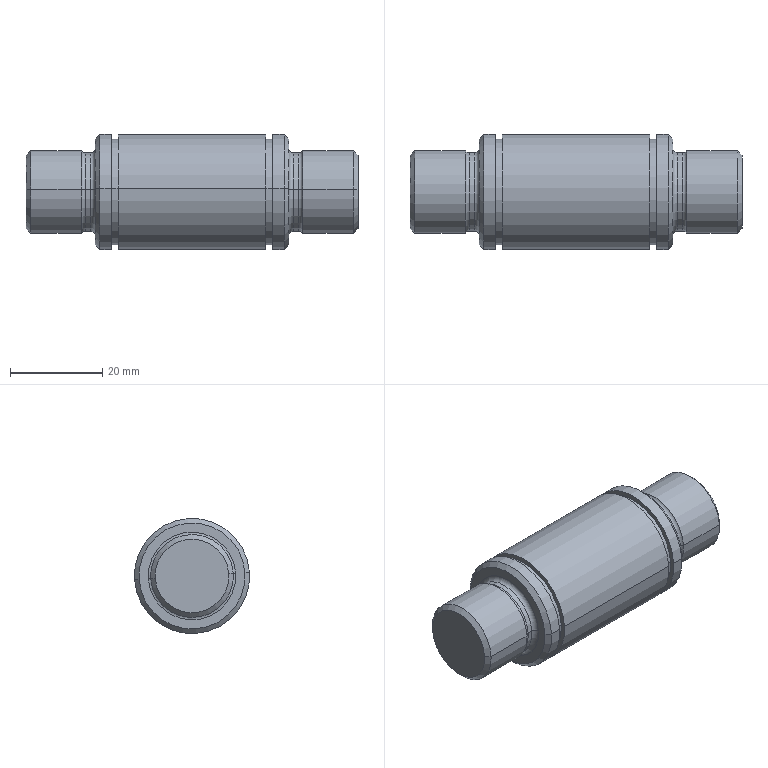Part | NX | features BREP 1 | 1 solid | 42 faces | box 72 x 25 x 25 mm | volume 27766 mm3 | cylinder 18 | cone 8 | torus 8 | plane 8 | commonest cylinder face diameters 25 x6 17 x4 18 x4 23 x4
STEP:
#1=CARTESIAN_POINT('',(-570.855,-69.053,-19.134));
#2=VERTEX_POINT('',#1);
#3=CARTESIAN_POINT('',(-570.855,-44.108,-20.797));
#4=VERTEX_POINT('',#3);
#5=CARTESIAN_POINT('',(-570.855,-56.581,-19.965));
#6=DIRECTION('',(1.,0.,0.));
#7=DIRECTION('',(0.,0.9978,-0.06652));
#8=AXIS2_PLACEMENT_3D('',#5,#6,#7);
#9=CIRCLE('',#8,12.5);
#10=EDGE_CURVE('',#2,#4,#9,.T.);
#11=ORIENTED_EDGE('',*,*,#10,.T.);
#12=CARTESIAN_POINT('',(-568.355,-44.108,-20.797));
#13=VERTEX_POINT('',#12);
#14=CARTESIAN_POINT('',(-609.355,-44.108,-20.797));
#15=DIRECTION('',(1.,0.,0.));
#16=VECTOR('',#15,1000.);
#17=LINE('',#14,#16);
#18=EDGE_CURVE('',#13,#4,#17,.F.);
#19=ORIENTED_EDGE('',*,*,#18,.F.);
#20=CARTESIAN_POINT('',(-568.355,-69.053,-19.134));
#21=VERTEX_POINT('',#20);
#22=CARTESIAN_POINT('',(-568.355,-56.581,-19.965));
#23=DIRECTION('',(-1.,0.,0.));
#24=DIRECTION('',(0.,-0.9978,0.06652));
#25=AXIS2_PLACEMENT_3D('',#22,#23,#24);
#26=CIRCLE('',#25,12.5);
#27=EDGE_CURVE('',#13,#21,#26,.T.);
#28=ORIENTED_EDGE('',*,*,#27,.T.);
#29=CARTESIAN_POINT('',(-609.355,-69.053,-19.134));
#30=DIRECTION('',(1.,0.,0.));
#31=VECTOR('',#30,1000.);
#32=LINE('',#29,#31);
#33=EDGE_CURVE('',#21,#2,#32,.F.);
#34=ORIENTED_EDGE('',*,*,#33,.T.);
#35=EDGE_LOOP('',(#11,#19,#28,#34));
#36=FACE_BOUND('',#35,.T.);
#37=CARTESIAN_POINT('',(-609.355,-56.581,-19.965));
#38=DIRECTION('',(1.,0.,0.));
#39=DIRECTION('',(0.,0.9978,-0.06652));
#40=AXIS2_PLACEMENT_3D('',#37,#38,#39);
#41=CYLINDRICAL_SURFACE('',#40,12.5);
#42=ADVANCED_FACE('',(#36),#41,.T.);
#43=CARTESIAN_POINT('',(-567.355,-68.055,-19.2));
#44=VERTEX_POINT('',#43);
#45=CARTESIAN_POINT('',(-567.355,-45.106,-20.73));
#46=VERTEX_POINT('',#45);
#47=CARTESIAN_POINT('',(-567.355,-56.581,-19.965));
#48=DIRECTION('',(1.,0.,0.));
#49=DIRECTION('',(0.,-0.9978,0.06652));
#50=AXIS2_PLACEMENT_3D('',#47,#48,#49);
#51=CIRCLE('',#50,11.5);
#52=EDGE_CURVE('',#44,#46,#51,.T.);
#53=ORIENTED_EDGE('',*,*,#52,.F.);
#54=CARTESIAN_POINT('',(-568.355,-69.053,-19.134));
#55=DIRECTION('',(-0.7071,-0.7055,0.04704));
#56=VECTOR('',#55,1000.);
#57=LINE('',#54,#56);
#58=EDGE_CURVE('',#44,#21,#57,.T.);
#59=ORIENTED_EDGE('',*,*,#58,.T.);
#60=ORIENTED_EDGE('',*,*,#27,.F.);
#61=CARTESIAN_POINT('',(-568.355,-44.108,-20.797));
#62=DIRECTION('',(-0.7071,0.7055,-0.04704));
#63=VECTOR('',#62,1000.);
#64=LINE('',#61,#63);
#65=EDGE_CURVE('',#46,#13,#64,.T.);
#66=ORIENTED_EDGE('',*,*,#65,.F.);
#67=EDGE_LOOP('',(#53,#59,#60,#66));
#68=FACE_BOUND('',#67,.T.);
#69=CARTESIAN_POINT('',(-568.355,-56.581,-19.965));
#70=DIRECTION('',(-1.,0.,0.));
#71=DIRECTION('',(0.,-0.9978,0.06652));
#72=AXIS2_PLACEMENT_3D('',#69,#70,#71);
#73=CONICAL_SURFACE('',#72,12.5,0.7854);
#74=ADVANCED_FACE('',(#68),#73,.T.);
#75=CARTESIAN_POINT('',(-565.221,-48.1,-20.531));
#76=VERTEX_POINT('',#75);
#77=CARTESIAN_POINT('',(-565.221,-65.062,-19.4));
#78=VERTEX_POINT('',#77);
#79=CARTESIAN_POINT('',(-565.221,-56.581,-19.965));
#80=DIRECTION('',(-1.,0.,0.));
#81=DIRECTION('',(0.,0.9978,-0.06652));
#82=AXIS2_PLACEMENT_3D('',#79,#80,#81);
#83=CIRCLE('',#82,8.5);
#84=EDGE_CURVE('',#76,#78,#83,.T.);
#85=ORIENTED_EDGE('',*,*,#84,.T.);
#86=CARTESIAN_POINT('',(-566.355,-65.062,-19.4));
#87=VERTEX_POINT('',#86);
#88=CARTESIAN_POINT('',(-564.355,-65.062,-19.4));
#89=DIRECTION('',(-1.,0.,0.));
#90=VECTOR('',#89,1000.);
#91=LINE('',#88,#90);
#92=EDGE_CURVE('',#78,#87,#91,.T.);
#93=ORIENTED_EDGE('',*,*,#92,.T.);
#94=CARTESIAN_POINT('',(-566.355,-48.1,-20.531));
#95=VERTEX_POINT('',#94);
#96=CARTESIAN_POINT('',(-566.355,-56.581,-19.965));
#97=DIRECTION('',(1.,0.,0.));
#98=DIRECTION('',(0.,-0.9978,0.06652));
#99=AXIS2_PLACEMENT_3D('',#96,#97,#98);
#100=CIRCLE('',#99,8.5);
#101=EDGE_CURVE('',#87,#95,#100,.T.);
#102=ORIENTED_EDGE('',*,*,#101,.T.);
#103=CARTESIAN_POINT('',(-564.355,-48.1,-20.531));
#104=DIRECTION('',(-1.,0.,0.));
#105=VECTOR('',#104,1000.);
#106=LINE('',#103,#105);
#107=EDGE_CURVE('',#76,#95,#106,.T.);
#108=ORIENTED_EDGE('',*,*,#107,.F.);
#109=EDGE_LOOP('',(#85,#93,#102,#108));
#110=FACE_BOUND('',#109,.T.);
#111=CARTESIAN_POINT('',(-564.355,-56.581,-19.965));
#112=DIRECTION('',(-1.,0.,0.));
#113=DIRECTION('',(0.,-0.9978,0.06652));
#114=AXIS2_PLACEMENT_3D('',#111,#112,#113);
#115=CYLINDRICAL_SURFACE('',#114,8.5);
#116=ADVANCED_FACE('',(#110),#115,.T.);
#117=CARTESIAN_POINT('',(-553.355,-47.601,-20.564));
#118=VERTEX_POINT('',#117);
#119=CARTESIAN_POINT('',(-553.355,-65.561,-19.367));
#120=VERTEX_POINT('',#119);
#121=CARTESIAN_POINT('',(-553.355,-56.581,-19.965));
#122=DIRECTION('',(-1.,0.,0.));
#123=DIRECTION('',(0.,0.9978,-0.06652));
#124=AXIS2_PLACEMENT_3D('',#121,#122,#123);
#125=CIRCLE('',#124,9.);
#126=EDGE_CURVE('',#118,#120,#125,.T.);
#127=ORIENTED_EDGE('',*,*,#126,.T.);
#128=CARTESIAN_POINT('',(-564.355,-65.561,-19.367));
#129=VERTEX_POINT('',#128);
#130=CARTESIAN_POINT('',(-552.355,-65.561,-19.367));
#131=DIRECTION('',(-1.,0.,0.));
#132=VECTOR('',#131,1000.);
#133=LINE('',#130,#132);
#134=EDGE_CURVE('',#120,#129,#133,.T.);
#135=ORIENTED_EDGE('',*,*,#134,.T.);
#136=CARTESIAN_POINT('',(-564.355,-47.601,-20.564));
#137=VERTEX_POINT('',#136);
#138=CARTESIAN_POINT('',(-564.355,-56.581,-19.965));
#139=DIRECTION('',(1.,0.,0.));
#140=DIRECTION('',(0.,0.9978,-0.06652));
#141=AXIS2_PLACEMENT_3D('',#138,#139,#140);
#142=CIRCLE('',#141,9.);
#143=EDGE_CURVE('',#129,#137,#142,.T.);
#144=ORIENTED_EDGE('',*,*,#143,.T.);
#145=CARTESIAN_POINT('',(-552.355,-47.601,-20.564));
#146=DIRECTION('',(-1.,0.,0.));
#147=VECTOR('',#146,1000.);
#148=LINE('',#145,#147);
#149=EDGE_CURVE('',#118,#137,#148,.T.);
#150=ORIENTED_EDGE('',*,*,#149,.F.);
#151=EDGE_LOOP('',(#127,#135,#144,#150));
#152=FACE_BOUND('',#151,.T.);
#153=CARTESIAN_POINT('',(-552.355,-56.581,-19.965));
#154=DIRECTION('',(-1.,0.,0.));
#155=DIRECTION('',(0.,-0.9978,0.06652));
#156=AXIS2_PLACEMENT_3D('',#153,#154,#155);
#157=CYLINDRICAL_SURFACE('',#156,9.);
#158=ADVANCED_FACE('',(#152),#157,.T.);
#159=CARTESIAN_POINT('',(-552.355,-64.563,-19.433));
#160=VERTEX_POINT('',#159);
#161=CARTESIAN_POINT('',(-552.355,-48.598,-20.498));
#162=VERTEX_POINT('',#161);
#163=CARTESIAN_POINT('',(-552.355,-56.581,-19.965));
#164=DIRECTION('',(1.,0.,0.));
#165=DIRECTION('',(0.,0.9978,-0.06652));
#166=AXIS2_PLACEMENT_3D('',#163,#164,#165);
#167=CIRCLE('',#166,8.);
#168=EDGE_CURVE('',#160,#162,#167,.T.);
#169=ORIENTED_EDGE('',*,*,#168,.F.);
#170=CARTESIAN_POINT('',(-552.355,-64.563,-19.433));
#171=DIRECTION('',(-0.7071,-0.7055,0.04704));
#172=VECTOR('',#171,1000.);
#173=LINE('',#170,#172);
#174=EDGE_CURVE('',#160,#120,#173,.T.);
#175=ORIENTED_EDGE('',*,*,#174,.T.);
#176=ORIENTED_EDGE('',*,*,#126,.F.);
#177=CARTESIAN_POINT('',(-552.355,-48.598,-20.498));
#178=DIRECTION('',(-0.7071,0.7055,-0.04704));
#179=VECTOR('',#178,1000.);
#180=LINE('',#177,#179);
#181=EDGE_CURVE('',#162,#118,#180,.T.);
#182=ORIENTED_EDGE('',*,*,#181,.F.);
#183=EDGE_LOOP('',(#169,#175,#176,#182));
#184=FACE_BOUND('',#183,.T.);
#185=CARTESIAN_POINT('',(-552.355,-56.581,-19.965));
#186=DIRECTION('',(-1.,0.,0.));
#187=DIRECTION('',(0.,-0.9978,0.06652));
#188=AXIS2_PLACEMENT_3D('',#185,#186,#187);
#189=CONICAL_SURFACE('',#188,8.,0.7854);
#190=ADVANCED_FACE('',(#184),#189,.T.);
#191=CARTESIAN_POINT('',(-572.355,-68.055,-19.2));
#192=VERTEX_POINT('',#191);
#193=CARTESIAN_POINT('',(-572.355,-45.106,-20.73));
#194=VERTEX_POINT('',#193);
#195=CARTESIAN_POINT('',(-572.355,-56.581,-19.965));
#196=DIRECTION('',(1.,0.,0.));
#197=DIRECTION('',(0.,0.9978,-0.06652));
#198=AXIS2_PLACEMENT_3D('',#195,#196,#197);
#199=CIRCLE('',#198,11.5);
#200=EDGE_CURVE('',#192,#194,#199,.T.);
#201=ORIENTED_EDGE('',*,*,#200,.T.);
#202=CARTESIAN_POINT('',(-570.855,-45.106,-20.73));
#203=VERTEX_POINT('',#202);
#204=CARTESIAN_POINT('',(-572.355,-45.106,-20.73));
#205=DIRECTION('',(1.,0.,0.));
#206=VECTOR('',#205,1000.);
#207=LINE('',#204,#206);
#208=EDGE_CURVE('',#203,#194,#207,.F.);
#209=ORIENTED_EDGE('',*,*,#208,.F.);
#210=CARTESIAN_POINT('',(-570.855,-68.055,-19.2));
#211=VERTEX_POINT('',#210);
#212=CARTESIAN_POINT('',(-570.855,-56.581,-19.965));
#213=DIRECTION('',(1.,0.,0.));
#214=DIRECTION('',(0.,0.9978,-0.06652));
#215=AXIS2_PLACEMENT_3D('',#212,#213,#214);
#216=CIRCLE('',#215,11.5);
#217=EDGE_CURVE('',#211,#203,#216,.T.);
#218=ORIENTED_EDGE('',*,*,#217,.F.);
#219=CARTESIAN_POINT('',(-572.355,-68.055,-19.2));
#220=DIRECTION('',(1.,0.,0.));
#221=VECTOR('',#220,1000.);
#222=LINE('',#219,#221);
#223=EDGE_CURVE('',#211,#192,#222,.F.);
#224=ORIENTED_EDGE('',*,*,#223,.T.);
#225=EDGE_LOOP('',(#201,#209,#218,#224));
#226=FACE_BOUND('',#225,.T.);
#227=CARTESIAN_POINT('',(-572.355,-56.581,-19.965));
#228=DIRECTION('',(1.,0.,0.));
#229=DIRECTION('',(0.,0.9978,-0.06652));
#230=AXIS2_PLACEMENT_3D('',#227,#228,#229);
#231=CYLINDRICAL_SURFACE('',#230,11.5);
#232=ADVANCED_FACE('',(#226),#231,.T.);
#233=CARTESIAN_POINT('',(-608.355,-69.053,-19.134));
#234=VERTEX_POINT('',#233);
#235=CARTESIAN_POINT('',(-608.355,-44.108,-20.797));
#236=VERTEX_POINT('',#235);
#237=CARTESIAN_POINT('',(-608.355,-56.581,-19.965));
#238=DIRECTION('',(1.,0.,0.));
#239=DIRECTION('',(0.,-0.9978,0.06652));
#240=AXIS2_PLACEMENT_3D('',#237,#238,#239);
#241=CIRCLE('',#240,12.5);
#242=EDGE_CURVE('',#234,#236,#241,.T.);
#243=ORIENTED_EDGE('',*,*,#242,.T.);
#244=CARTESIAN_POINT('',(-605.855,-44.108,-20.797));
#245=VERTEX_POINT('',#244);
#246=CARTESIAN_POINT('',(-609.355,-44.108,-20.797));
#247=DIRECTION('',(1.,0.,0.));
#248=VECTOR('',#247,1000.);
#249=LINE('',#246,#248);
#250=EDGE_CURVE('',#245,#236,#249,.F.);
#251=ORIENTED_EDGE('',*,*,#250,.F.);
#252=CARTESIAN_POINT('',(-605.855,-69.053,-19.134));
#253=VERTEX_POINT('',#252);
#254=CARTESIAN_POINT('',(-605.855,-56.581,-19.965));
#255=DIRECTION('',(-1.,0.,0.));
#256=DIRECTION('',(0.,-0.9978,0.06652));
#257=AXIS2_PLACEMENT_3D('',#254,#255,#256);
#258=CIRCLE('',#257,12.5);
#259=EDGE_CURVE('',#245,#253,#258,.T.);
#260=ORIENTED_EDGE('',*,*,#259,.T.);
#261=CARTESIAN_POINT('',(-609.355,-69.053,-19.134));
#262=DIRECTION('',(1.,0.,0.));
#263=VECTOR('',#262,1000.);
#264=LINE('',#261,#263);
#265=EDGE_CURVE('',#253,#234,#264,.F.);
#266=ORIENTED_EDGE('',*,*,#265,.T.);
#267=EDGE_LOOP('',(#243,#251,#260,#266));
#268=FACE_BOUND('',#267,.T.);
#269=CARTESIAN_POINT('',(-609.355,-56.581,-19.965));
#270=DIRECTION('',(1.,0.,0.));
#271=DIRECTION('',(0.,0.9978,-0.06652));
#272=AXIS2_PLACEMENT_3D('',#269,#270,#271);
#273=CYLINDRICAL_SURFACE('',#272,12.5);
#274=ADVANCED_FACE('',(#268),#273,.T.);
#275=CARTESIAN_POINT('',(-609.355,-45.106,-20.73));
#276=VERTEX_POINT('',#275);
#277=CARTESIAN_POINT('',(-609.355,-68.055,-19.2));
#278=VERTEX_POINT('',#277);
#279=CARTESIAN_POINT('',(-609.355,-56.581,-19.965));
#280=DIRECTION('',(-1.,0.,0.));
#281=DIRECTION('',(0.,-0.9978,0.06652));
#282=AXIS2_PLACEMENT_3D('',#279,#280,#281);
#283=CIRCLE('',#282,11.5);
#284=EDGE_CURVE('',#276,#278,#283,.T.);
#285=ORIENTED_EDGE('',*,*,#284,.F.);
#286=CARTESIAN_POINT('',(-609.355,-45.106,-20.73));
#287=DIRECTION('',(0.7071,0.7055,-0.04704));
#288=VECTOR('',#287,1000.);
#289=LINE('',#286,#288);
#290=EDGE_CURVE('',#236,#276,#289,.F.);
#291=ORIENTED_EDGE('',*,*,#290,.F.);
#292=ORIENTED_EDGE('',*,*,#242,.F.);
#293=CARTESIAN_POINT('',(-609.355,-68.055,-19.2));
#294=DIRECTION('',(0.7071,-0.7055,0.04704));
#295=VECTOR('',#294,1000.);
#296=LINE('',#293,#295);
#297=EDGE_CURVE('',#234,#278,#296,.F.);
#298=ORIENTED_EDGE('',*,*,#297,.T.);
#299=EDGE_LOOP('',(#285,#291,#292,#298));
#300=FACE_BOUND('',#299,.T.);
#301=CARTESIAN_POINT('',(-609.355,-56.581,-19.965));
#302=DIRECTION('',(1.,0.,0.));
#303=DIRECTION('',(0.,0.9978,-0.06652));
#304=AXIS2_PLACEMENT_3D('',#301,#302,#303);
#305=CONICAL_SURFACE('',#304,11.5,0.7854);
#306=ADVANCED_FACE('',(#300),#305,.T.);
#307=CARTESIAN_POINT('',(-611.489,-65.062,-19.4));
#308=VERTEX_POINT('',#307);
#309=CARTESIAN_POINT('',(-611.489,-48.1,-20.531));
#310=VERTEX_POINT('',#309);
#311=CARTESIAN_POINT('',(-611.489,-56.581,-19.965));
#312=DIRECTION('',(1.,0.,0.));
#313=DIRECTION('',(0.,-0.9978,0.06652));
#314=AXIS2_PLACEMENT_3D('',#311,#312,#313);
#315=CIRCLE('',#314,8.5);
#316=EDGE_CURVE('',#308,#310,#315,.T.);
#317=ORIENTED_EDGE('',*,*,#316,.T.);
#318=CARTESIAN_POINT('',(-610.355,-48.1,-20.531));
#319=VERTEX_POINT('',#318);
#320=CARTESIAN_POINT('',(-612.355,-48.1,-20.531));
#321=DIRECTION('',(1.,0.,0.));
#322=VECTOR('',#321,1000.);
#323=LINE('',#320,#322);
#324=EDGE_CURVE('',#319,#310,#323,.F.);
#325=ORIENTED_EDGE('',*,*,#324,.F.);
#326=CARTESIAN_POINT('',(-610.355,-65.062,-19.4));
#327=VERTEX_POINT('',#326);
#328=CARTESIAN_POINT('',(-610.355,-56.581,-19.965));
#329=DIRECTION('',(-1.,0.,0.));
#330=DIRECTION('',(0.,-0.9978,0.06652));
#331=AXIS2_PLACEMENT_3D('',#328,#329,#330);
#332=CIRCLE('',#331,8.5);
#333=EDGE_CURVE('',#319,#327,#332,.T.);
#334=ORIENTED_EDGE('',*,*,#333,.T.);
#335=CARTESIAN_POINT('',(-612.355,-65.062,-19.4));
#336=DIRECTION('',(1.,0.,0.));
#337=VECTOR('',#336,1000.);
#338=LINE('',#335,#337);
#339=EDGE_CURVE('',#327,#308,#338,.F.);
#340=ORIENTED_EDGE('',*,*,#339,.T.);
#341=EDGE_LOOP('',(#317,#325,#334,#340));
#342=FACE_BOUND('',#341,.T.);
#343=CARTESIAN_POINT('',(-612.355,-56.581,-19.965));
#344=DIRECTION('',(1.,0.,0.));
#345=DIRECTION('',(0.,0.9978,-0.06652));
#346=AXIS2_PLACEMENT_3D('',#343,#344,#345);
#347=CYLINDRICAL_SURFACE('',#346,8.5);
#348=ADVANCED_FACE('',(#342),#347,.T.);
#349=CARTESIAN_POINT('',(-623.355,-65.561,-19.367));
#350=VERTEX_POINT('',#349);
#351=CARTESIAN_POINT('',(-623.355,-47.601,-20.564));
#352=VERTEX_POINT('',#351);
#353=CARTESIAN_POINT('',(-623.355,-56.581,-19.965));
#354=DIRECTION('',(1.,0.,0.));
#355=DIRECTION('',(0.,-0.9978,0.06652));
#356=AXIS2_PLACEMENT_3D('',#353,#354,#355);
#357=CIRCLE('',#356,9.);
#358=EDGE_CURVE('',#350,#352,#357,.T.);
#359=ORIENTED_EDGE('',*,*,#358,.T.);
#360=CARTESIAN_POINT('',(-612.355,-47.601,-20.564));
#361=VERTEX_POINT('',#360);
#362=CARTESIAN_POINT('',(-624.355,-47.601,-20.564));
#363=DIRECTION('',(1.,0.,0.));
#364=VECTOR('',#363,1000.);
#365=LINE('',#362,#364);
#366=EDGE_CURVE('',#361,#352,#365,.F.);
#367=ORIENTED_EDGE('',*,*,#366,.F.);
#368=CARTESIAN_POINT('',(-612.355,-65.561,-19.367));
#369=VERTEX_POINT('',#368);
#370=CARTESIAN_POINT('',(-612.355,-56.581,-19.965));
#371=DIRECTION('',(-1.,0.,0.));
#372=DIRECTION('',(0.,-0.9978,0.06652));
#373=AXIS2_PLACEMENT_3D('',#370,#371,#372);
#374=CIRCLE('',#373,9.);
#375=EDGE_CURVE('',#361,#369,#374,.T.);
#376=ORIENTED_EDGE('',*,*,#375,.T.);
#377=CARTESIAN_POINT('',(-624.355,-65.561,-19.367));
#378=DIRECTION('',(1.,0.,0.));
#379=VECTOR('',#378,1000.);
#380=LINE('',#377,#379);
#381=EDGE_CURVE('',#369,#350,#380,.F.);
#382=ORIENTED_EDGE('',*,*,#381,.T.);
#383=EDGE_LOOP('',(#359,#367,#376,#382));
#384=FACE_BOUND('',#383,.T.);
#385=CARTESIAN_POINT('',(-624.355,-56.581,-19.965));
#386=DIRECTION('',(1.,0.,0.));
#387=DIRECTION('',(0.,0.9978,-0.06652));
#388=AXIS2_PLACEMENT_3D('',#385,#386,#387);
#389=CYLINDRICAL_SURFACE('',#388,9.);
#390=ADVANCED_FACE('',(#384),#389,.T.);
#391=CARTESIAN_POINT('',(-624.355,-48.598,-20.498));
#392=VERTEX_POINT('',#391);
#393=CARTESIAN_POINT('',(-624.355,-64.563,-19.433));
#394=VERTEX_POINT('',#393);
#395=CARTESIAN_POINT('',(-624.355,-56.581,-19.965));
#396=DIRECTION('',(-1.,0.,0.));
#397=DIRECTION('',(0.,-0.9978,0.06652));
#398=AXIS2_PLACEMENT_3D('',#395,#396,#397);
#399=CIRCLE('',#398,8.);
#400=EDGE_CURVE('',#392,#394,#399,.T.);
#401=ORIENTED_EDGE('',*,*,#400,.F.);
#402=CARTESIAN_POINT('',(-624.355,-48.598,-20.498));
#403=DIRECTION('',(0.7071,0.7055,-0.04704));
#404=VECTOR('',#403,1000.);
#405=LINE('',#402,#404);
#406=EDGE_CURVE('',#352,#392,#405,.F.);
#407=ORIENTED_EDGE('',*,*,#406,.F.);
#408=ORIENTED_EDGE('',*,*,#358,.F.);
#409=CARTESIAN_POINT('',(-624.355,-64.563,-19.433));
#410=DIRECTION('',(0.7071,-0.7055,0.04704));
#411=VECTOR('',#410,1000.);
#412=LINE('',#409,#411);
#413=EDGE_CURVE('',#350,#394,#412,.F.);
#414=ORIENTED_EDGE('',*,*,#413,.T.);
#415=EDGE_LOOP('',(#401,#407,#408,#414));
#416=FACE_BOUND('',#415,.T.);
#417=CARTESIAN_POINT('',(-624.355,-56.581,-19.965));
#418=DIRECTION('',(1.,0.,0.));
#419=DIRECTION('',(0.,0.9978,-0.06652));
#420=AXIS2_PLACEMENT_3D('',#417,#418,#419);
#421=CONICAL_SURFACE('',#420,8.,0.7854);
#422=ADVANCED_FACE('',(#416),#421,.T.);
#423=CARTESIAN_POINT('',(-604.355,-45.106,-20.73));
#424=VERTEX_POINT('',#423);
#425=CARTESIAN_POINT('',(-604.355,-68.055,-19.2));
#426=VERTEX_POINT('',#425);
#427=CARTESIAN_POINT('',(-604.355,-56.581,-19.965));
#428=DIRECTION('',(-1.,0.,0.));
#429=DIRECTION('',(0.,-0.9978,0.06652));
#430=AXIS2_PLACEMENT_3D('',#427,#428,#429);
#431=CIRCLE('',#430,11.5);
#432=EDGE_CURVE('',#424,#426,#431,.T.);
#433=ORIENTED_EDGE('',*,*,#432,.T.);
#434=CARTESIAN_POINT('',(-605.855,-68.055,-19.2));
#435=VERTEX_POINT('',#434);
#436=CARTESIAN_POINT('',(-604.355,-68.055,-19.2));
#437=DIRECTION('',(-1.,0.,0.));
#438=VECTOR('',#437,1000.);
#439=LINE('',#436,#438);
#440=EDGE_CURVE('',#426,#435,#439,.T.);
#441=ORIENTED_EDGE('',*,*,#440,.T.);
#442=CARTESIAN_POINT('',(-605.855,-45.106,-20.73));
#443=VERTEX_POINT('',#442);
#444=CARTESIAN_POINT('',(-605.855,-56.581,-19.965));
#445=DIRECTION('',(-1.,0.,0.));
#446=DIRECTION('',(0.,-0.9978,0.06652));
#447=AXIS2_PLACEMENT_3D('',#444,#445,#446);
#448=CIRCLE('',#447,11.5);
#449=EDGE_CURVE('',#443,#435,#448,.T.);
#450=ORIENTED_EDGE('',*,*,#449,.F.);
#451=CARTESIAN_POINT('',(-604.355,-45.106,-20.73));
#452=DIRECTION('',(-1.,0.,0.));
#453=VECTOR('',#452,1000.);
#454=LINE('',#451,#453);
#455=EDGE_CURVE('',#424,#443,#454,.T.);
#456=ORIENTED_EDGE('',*,*,#455,.F.);
#457=EDGE_LOOP('',(#433,#441,#450,#456));
#458=FACE_BOUND('',#457,.T.);
#459=CARTESIAN_POINT('',(-604.355,-56.581,-19.965));
#460=DIRECTION('',(-1.,0.,0.));
#461=DIRECTION('',(0.,-0.9978,0.06652));
#462=AXIS2_PLACEMENT_3D('',#459,#460,#461);
#463=CYLINDRICAL_SURFACE('',#462,11.5);
#464=ADVANCED_FACE('',(#458),#463,.T.);
#465=CARTESIAN_POINT('',(-604.355,-44.108,-20.797));
#466=VERTEX_POINT('',#465);
#467=CARTESIAN_POINT('',(-604.355,-69.053,-19.134));
#468=VERTEX_POINT('',#467);
#469=CARTESIAN_POINT('',(-604.355,-56.581,-19.965));
#470=DIRECTION('',(-1.,0.,0.));
#471=DIRECTION('',(0.,-0.9978,0.06652));
#472=AXIS2_PLACEMENT_3D('',#469,#470,#471);
#473=CIRCLE('',#472,12.5);
#474=EDGE_CURVE('',#466,#468,#473,.T.);
#475=ORIENTED_EDGE('',*,*,#474,.F.);
#476=CARTESIAN_POINT('',(-572.355,-44.108,-20.797));
#477=VERTEX_POINT('',#476);
#478=CARTESIAN_POINT('',(-609.355,-44.108,-20.797));
#479=DIRECTION('',(1.,0.,0.));
#480=VECTOR('',#479,1000.);
#481=LINE('',#478,#480);
#482=EDGE_CURVE('',#477,#466,#481,.F.);
#483=ORIENTED_EDGE('',*,*,#482,.F.);
#484=CARTESIAN_POINT('',(-572.355,-69.053,-19.134));
#485=VERTEX_POINT('',#484);
#486=CARTESIAN_POINT('',(-572.355,-56.581,-19.965));
#487=DIRECTION('',(1.,0.,0.));
#488=DIRECTION('',(0.,0.9978,-0.06652));
#489=AXIS2_PLACEMENT_3D('',#486,#487,#488);
#490=CIRCLE('',#489,12.5);
#491=EDGE_CURVE('',#485,#477,#490,.T.);
#492=ORIENTED_EDGE('',*,*,#491,.F.);
#493=CARTESIAN_POINT('',(-609.355,-69.053,-19.134));
#494=DIRECTION('',(1.,0.,0.));
#495=VECTOR('',#494,1000.);
#496=LINE('',#493,#495);
#497=EDGE_CURVE('',#485,#468,#496,.F.);
#498=ORIENTED_EDGE('',*,*,#497,.T.);
#499=EDGE_LOOP('',(#475,#483,#492,#498));
#500=FACE_BOUND('',#499,.T.);
#501=CARTESIAN_POINT('',(-609.355,-56.581,-19.965));
#502=DIRECTION('',(1.,0.,0.));
#503=DIRECTION('',(0.,0.9978,-0.06652));
#504=AXIS2_PLACEMENT_3D('',#501,#502,#503);
#505=CYLINDRICAL_SURFACE('',#504,12.5);
#506=ADVANCED_FACE('',(#500),#505,.T.);
#507=CARTESIAN_POINT('',(-612.355,-56.581,-19.965));
#508=DIRECTION('',(-1.,0.,0.));
#509=DIRECTION('',(0.,-0.9978,0.06652));
#510=AXIS2_PLACEMENT_3D('',#507,#508,#509);
#511=CIRCLE('',#510,9.);
#512=EDGE_CURVE('',#369,#361,#511,.T.);
#513=ORIENTED_EDGE('',*,*,#512,.F.);
#514=CARTESIAN_POINT('',(-611.489,-66.06,-19.333));
#515=DIRECTION('',(0.,-0.06652,-0.9978));
#516=DIRECTION('',(0.,0.9978,-0.06652));
#517=AXIS2_PLACEMENT_3D('',#514,#515,#516);
#518=CIRCLE('',#517,1.);
#519=EDGE_CURVE('',#369,#308,#518,.T.);
#520=ORIENTED_EDGE('',*,*,#519,.T.);
#521=CARTESIAN_POINT('',(-611.489,-56.581,-19.965));
#522=DIRECTION('',(1.,0.,0.));
#523=DIRECTION('',(0.,-0.9978,0.06652));
#524=AXIS2_PLACEMENT_3D('',#521,#522,#523);
#525=CIRCLE('',#524,8.5);
#526=EDGE_CURVE('',#310,#308,#525,.T.);
#527=ORIENTED_EDGE('',*,*,#526,.F.);
#528=CARTESIAN_POINT('',(-611.489,-47.102,-20.597));
#529=DIRECTION('',(0.,0.06652,0.9978));
#530=DIRECTION('',(0.,-0.9978,0.06652));
#531=AXIS2_PLACEMENT_3D('',#528,#529,#530);
#532=CIRCLE('',#531,1.);
#533=EDGE_CURVE('',#361,#310,#532,.T.);
#534=ORIENTED_EDGE('',*,*,#533,.F.);
#535=EDGE_LOOP('',(#513,#520,#527,#534));
#536=FACE_BOUND('',#535,.T.);
#537=CARTESIAN_POINT('',(-611.489,-56.581,-19.965));
#538=DIRECTION('',(-1.,0.,0.));
#539=DIRECTION('',(0.,-0.9978,0.06652));
#540=AXIS2_PLACEMENT_3D('',#537,#538,#539);
#541=TOROIDAL_SURFACE('',#540,9.5,1.);
#542=ADVANCED_FACE('',(#536),#541,.F.);
#543=CARTESIAN_POINT('',(-610.355,-56.581,-19.965));
#544=DIRECTION('',(-1.,0.,0.));
#545=DIRECTION('',(0.,-0.9978,0.06652));
#546=AXIS2_PLACEMENT_3D('',#543,#544,#545);
#547=CIRCLE('',#546,8.5);
#548=EDGE_CURVE('',#327,#319,#547,.T.);
#549=ORIENTED_EDGE('',*,*,#548,.F.);
#550=CARTESIAN_POINT('',(-609.355,-66.06,-19.333));
#551=VERTEX_POINT('',#550);
#552=CARTESIAN_POINT('',(-610.355,-66.06,-19.333));
#553=DIRECTION('',(0.,-0.06652,-0.9978));
#554=DIRECTION('',(0.,0.9978,-0.06652));
#555=AXIS2_PLACEMENT_3D('',#552,#553,#554);
#556=CIRCLE('',#555,1.);
#557=EDGE_CURVE('',#327,#551,#556,.T.);
#558=ORIENTED_EDGE('',*,*,#557,.T.);
#559=CARTESIAN_POINT('',(-609.355,-47.102,-20.597));
#560=VERTEX_POINT('',#559);
#561=CARTESIAN_POINT('',(-609.355,-56.581,-19.965));
#562=DIRECTION('',(1.,0.,0.));
#563=DIRECTION('',(0.,-0.9978,0.06652));
#564=AXIS2_PLACEMENT_3D('',#561,#562,#563);
#565=CIRCLE('',#564,9.5);
#566=EDGE_CURVE('',#560,#551,#565,.T.);
#567=ORIENTED_EDGE('',*,*,#566,.F.);
#568=CARTESIAN_POINT('',(-610.355,-47.102,-20.597));
#569=DIRECTION('',(0.,0.06652,0.9978));
#570=DIRECTION('',(0.,-0.9978,0.06652));
#571=AXIS2_PLACEMENT_3D('',#568,#569,#570);
#572=CIRCLE('',#571,1.);
#573=EDGE_CURVE('',#319,#560,#572,.T.);
#574=ORIENTED_EDGE('',*,*,#573,.F.);
#575=EDGE_LOOP('',(#549,#558,#567,#574));
#576=FACE_BOUND('',#575,.T.);
#577=CARTESIAN_POINT('',(-610.355,-56.581,-19.965));
#578=DIRECTION('',(-1.,0.,0.));
#579=DIRECTION('',(0.,-0.9978,0.06652));
#580=AXIS2_PLACEMENT_3D('',#577,#578,#579);
#581=TOROIDAL_SURFACE('',#580,9.5,1.);
#582=ADVANCED_FACE('',(#576),#581,.F.);
#583=CARTESIAN_POINT('',(-564.355,-56.581,-19.965));
#584=DIRECTION('',(1.,0.,0.));
#585=DIRECTION('',(0.,0.9978,-0.06652));
#586=AXIS2_PLACEMENT_3D('',#583,#584,#585);
#587=CIRCLE('',#586,9.);
#588=EDGE_CURVE('',#137,#129,#587,.T.);
#589=ORIENTED_EDGE('',*,*,#588,.F.);
#590=CARTESIAN_POINT('',(-565.221,-47.102,-20.597));
#591=DIRECTION('',(0.,-0.06652,-0.9978));
#592=DIRECTION('',(0.,0.9978,-0.06652));
#593=AXIS2_PLACEMENT_3D('',#590,#591,#592);
#594=CIRCLE('',#593,1.);
#595=EDGE_CURVE('',#76,#137,#594,.F.);
#596=ORIENTED_EDGE('',*,*,#595,.F.);
#597=CARTESIAN_POINT('',(-565.221,-56.581,-19.965));
#598=DIRECTION('',(-1.,0.,0.));
#599=DIRECTION('',(0.,0.9978,-0.06652));
#600=AXIS2_PLACEMENT_3D('',#597,#598,#599);
#601=CIRCLE('',#600,8.5);
#602=EDGE_CURVE('',#78,#76,#601,.T.);
#603=ORIENTED_EDGE('',*,*,#602,.F.);
#604=CARTESIAN_POINT('',(-565.221,-66.06,-19.333));
#605=DIRECTION('',(0.,0.06652,0.9978));
#606=DIRECTION('',(0.,-0.9978,0.06652));
#607=AXIS2_PLACEMENT_3D('',#604,#605,#606);
#608=CIRCLE('',#607,1.);
#609=EDGE_CURVE('',#78,#129,#608,.F.);
#610=ORIENTED_EDGE('',*,*,#609,.T.);
#611=EDGE_LOOP('',(#589,#596,#603,#610));
#612=FACE_BOUND('',#611,.T.);
#613=CARTESIAN_POINT('',(-565.221,-56.581,-19.965));
#614=DIRECTION('',(1.,0.,0.));
#615=DIRECTION('',(0.,0.9978,-0.06652));
#616=AXIS2_PLACEMENT_3D('',#613,#614,#615);
#617=TOROIDAL_SURFACE('',#616,9.5,1.);
#618=ADVANCED_FACE('',(#612),#617,.F.);
#619=CARTESIAN_POINT('',(-567.355,-66.06,-19.333));
#620=VERTEX_POINT('',#619);
#621=CARTESIAN_POINT('',(-567.355,-47.102,-20.597));
#622=VERTEX_POINT('',#621);
#623=CARTESIAN_POINT('',(-567.355,-56.581,-19.965));
#624=DIRECTION('',(-1.,0.,0.));
#625=DIRECTION('',(0.,-0.9978,0.06652));
#626=AXIS2_PLACEMENT_3D('',#623,#624,#625);
#627=CIRCLE('',#626,9.5);
#628=EDGE_CURVE('',#620,#622,#627,.T.);
#629=ORIENTED_EDGE('',*,*,#628,.F.);
#630=CARTESIAN_POINT('',(-566.355,-66.06,-19.333));
#631=DIRECTION('',(0.,-0.06652,-0.9978));
#632=DIRECTION('',(0.,0.9978,-0.06652));
#633=AXIS2_PLACEMENT_3D('',#630,#631,#632);
#634=CIRCLE('',#633,1.);
#635=EDGE_CURVE('',#620,#87,#634,.T.);
#636=ORIENTED_EDGE('',*,*,#635,.T.);
#637=CARTESIAN_POINT('',(-566.355,-56.581,-19.965));
#638=DIRECTION('',(1.,0.,0.));
#639=DIRECTION('',(0.,-0.9978,0.06652));
#640=AXIS2_PLACEMENT_3D('',#637,#638,#639);
#641=CIRCLE('',#640,8.5);
#642=EDGE_CURVE('',#95,#87,#641,.T.);
#643=ORIENTED_EDGE('',*,*,#642,.F.);
#644=CARTESIAN_POINT('',(-566.355,-47.102,-20.597));
#645=DIRECTION('',(0.,0.06652,0.9978));
#646=DIRECTION('',(0.,-0.9978,0.06652));
#647=AXIS2_PLACEMENT_3D('',#644,#645,#646);
#648=CIRCLE('',#647,1.);
#649=EDGE_CURVE('',#622,#95,#648,.T.);
#650=ORIENTED_EDGE('',*,*,#649,.F.);
#651=EDGE_LOOP('',(#629,#636,#643,#650));
#652=FACE_BOUND('',#651,.T.);
#653=CARTESIAN_POINT('',(-566.355,-56.581,-19.965));
#654=DIRECTION('',(-1.,0.,0.));
#655=DIRECTION('',(0.,-0.9978,0.06652));
#656=AXIS2_PLACEMENT_3D('',#653,#654,#655);
#657=TOROIDAL_SURFACE('',#656,9.5,1.);
#658=ADVANCED_FACE('',(#652),#657,.F.);
#659=ORIENTED_EDGE('',*,*,#635,.F.);
#660=CARTESIAN_POINT('',(-567.355,-56.581,-19.965));
#661=DIRECTION('',(-1.,0.,0.));
#662=DIRECTION('',(0.,-0.9978,0.06652));
#663=AXIS2_PLACEMENT_3D('',#660,#661,#662);
#664=CIRCLE('',#663,9.5);
#665=EDGE_CURVE('',#622,#620,#664,.T.);
#666=ORIENTED_EDGE('',*,*,#665,.F.);
#667=ORIENTED_EDGE('',*,*,#649,.T.);
#668=ORIENTED_EDGE('',*,*,#101,.F.);
#669=EDGE_LOOP('',(#659,#666,#667,#668));
#670=FACE_BOUND('',#669,.T.);
#671=CARTESIAN_POINT('',(-566.355,-56.581,-19.965));
#672=DIRECTION('',(-1.,0.,0.));
#673=DIRECTION('',(0.,-0.9978,0.06652));
#674=AXIS2_PLACEMENT_3D('',#671,#672,#673);
#675=TOROIDAL_SURFACE('',#674,9.5,1.);
#676=ADVANCED_FACE('',(#670),#675,.F.);
#677=ORIENTED_EDGE('',*,*,#595,.T.);
#678=ORIENTED_EDGE('',*,*,#143,.F.);
#679=ORIENTED_EDGE('',*,*,#609,.F.);
#680=ORIENTED_EDGE('',*,*,#84,.F.);
#681=EDGE_LOOP('',(#677,#678,#679,#680));
#682=FACE_BOUND('',#681,.T.);
#683=CARTESIAN_POINT('',(-565.221,-56.581,-19.965));
#684=DIRECTION('',(1.,0.,0.));
#685=DIRECTION('',(0.,0.9978,-0.06652));
#686=AXIS2_PLACEMENT_3D('',#683,#684,#685);
#687=TOROIDAL_SURFACE('',#686,9.5,1.);
#688=ADVANCED_FACE('',(#682),#687,.F.);
#689=ORIENTED_EDGE('',*,*,#557,.F.);
#690=ORIENTED_EDGE('',*,*,#333,.F.);
#691=ORIENTED_EDGE('',*,*,#573,.T.);
#692=CARTESIAN_POINT('',(-609.355,-56.581,-19.965));
#693=DIRECTION('',(1.,0.,0.));
#694=DIRECTION('',(0.,-0.9978,0.06652));
#695=AXIS2_PLACEMENT_3D('',#692,#693,#694);
#696=CIRCLE('',#695,9.5);
#697=EDGE_CURVE('',#551,#560,#696,.T.);
#698=ORIENTED_EDGE('',*,*,#697,.F.);
#699=EDGE_LOOP('',(#689,#690,#691,#698));
#700=FACE_BOUND('',#699,.T.);
#701=CARTESIAN_POINT('',(-610.355,-56.581,-19.965));
#702=DIRECTION('',(-1.,0.,0.));
#703=DIRECTION('',(0.,-0.9978,0.06652));
#704=AXIS2_PLACEMENT_3D('',#701,#702,#703);
#705=TOROIDAL_SURFACE('',#704,9.5,1.);
#706=ADVANCED_FACE('',(#700),#705,.F.);
#707=ORIENTED_EDGE('',*,*,#519,.F.);
#708=ORIENTED_EDGE('',*,*,#375,.F.);
#709=ORIENTED_EDGE('',*,*,#533,.T.);
#710=ORIENTED_EDGE('',*,*,#316,.F.);
#711=EDGE_LOOP('',(#707,#708,#709,#710));
#712=FACE_BOUND('',#711,.T.);
#713=CARTESIAN_POINT('',(-611.489,-56.581,-19.965));
#714=DIRECTION('',(-1.,0.,0.));
#715=DIRECTION('',(0.,-0.9978,0.06652));
#716=AXIS2_PLACEMENT_3D('',#713,#714,#715);
#717=TOROIDAL_SURFACE('',#716,9.5,1.);
#718=ADVANCED_FACE('',(#712),#717,.F.);
#719=ORIENTED_EDGE('',*,*,#482,.T.);
#720=CARTESIAN_POINT('',(-604.355,-56.581,-19.965));
#721=DIRECTION('',(-1.,0.,0.));
#722=DIRECTION('',(0.,-0.9978,0.06652));
#723=AXIS2_PLACEMENT_3D('',#720,#721,#722);
#724=CIRCLE('',#723,12.5);
#725=EDGE_CURVE('',#468,#466,#724,.T.);
#726=ORIENTED_EDGE('',*,*,#725,.F.);
#727=ORIENTED_EDGE('',*,*,#497,.F.);
#728=CARTESIAN_POINT('',(-572.355,-56.581,-19.965));
#729=DIRECTION('',(1.,0.,0.));
#730=DIRECTION('',(0.,0.9978,-0.06652));
#731=AXIS2_PLACEMENT_3D('',#728,#729,#730);
#732=CIRCLE('',#731,12.5);
#733=EDGE_CURVE('',#477,#485,#732,.T.);
#734=ORIENTED_EDGE('',*,*,#733,.F.);
#735=EDGE_LOOP('',(#719,#726,#727,#734));
#736=FACE_BOUND('',#735,.T.);
#737=CARTESIAN_POINT('',(-609.355,-56.581,-19.965));
#738=DIRECTION('',(1.,0.,0.));
#739=DIRECTION('',(0.,0.9978,-0.06652));
#740=AXIS2_PLACEMENT_3D('',#737,#738,#739);
#741=CYLINDRICAL_SURFACE('',#740,12.5);
#742=ADVANCED_FACE('',(#736),#741,.T.);
#743=ORIENTED_EDGE('',*,*,#432,.F.);
#744=CARTESIAN_POINT('',(-604.355,-56.581,-19.965));
#745=DIRECTION('',(-1.,0.,0.));
#746=DIRECTION('',(0.,-0.9978,0.06652));
#747=AXIS2_PLACEMENT_3D('',#744,#745,#746);
#748=CIRCLE('',#747,11.5);
#749=EDGE_CURVE('',#426,#424,#748,.T.);
#750=ORIENTED_EDGE('',*,*,#749,.F.);
#751=EDGE_LOOP('',(#743,#750));
#752=FACE_BOUND('',#751,.T.);
#753=ORIENTED_EDGE('',*,*,#725,.T.);
#754=ORIENTED_EDGE('',*,*,#474,.T.);
#755=EDGE_LOOP('',(#753,#754));
#756=FACE_BOUND('',#755,.T.);
#757=CARTESIAN_POINT('',(-604.355,-56.581,-19.965));
#758=DIRECTION('',(-1.,0.,0.));
#759=DIRECTION('',(0.,-0.9978,0.06652));
#760=AXIS2_PLACEMENT_3D('',#757,#758,#759);
#761=PLANE('',#760);
#762=ADVANCED_FACE('',(#752,#756),#761,.T.);
#763=ORIENTED_EDGE('',*,*,#449,.T.);
#764=CARTESIAN_POINT('',(-605.855,-56.581,-19.965));
#765=DIRECTION('',(-1.,0.,0.));
#766=DIRECTION('',(0.,-0.9978,0.06652));
#767=AXIS2_PLACEMENT_3D('',#764,#765,#766);
#768=CIRCLE('',#767,11.5);
#769=EDGE_CURVE('',#435,#443,#768,.T.);
#770=ORIENTED_EDGE('',*,*,#769,.T.);
#771=EDGE_LOOP('',(#763,#770));
#772=FACE_BOUND('',#771,.T.);
#773=CARTESIAN_POINT('',(-605.855,-56.581,-19.965));
#774=DIRECTION('',(-1.,0.,0.));
#775=DIRECTION('',(0.,-0.9978,0.06652));
#776=AXIS2_PLACEMENT_3D('',#773,#774,#775);
#777=CIRCLE('',#776,12.5);
#778=EDGE_CURVE('',#253,#245,#777,.T.);
#779=ORIENTED_EDGE('',*,*,#778,.F.);
#780=ORIENTED_EDGE('',*,*,#259,.F.);
#781=EDGE_LOOP('',(#779,#780));
#782=FACE_BOUND('',#781,.T.);
#783=CARTESIAN_POINT('',(-605.855,-56.581,-19.965));
#784=DIRECTION('',(-1.,0.,0.));
#785=DIRECTION('',(0.,-0.9978,0.06652));
#786=AXIS2_PLACEMENT_3D('',#783,#784,#785);
#787=PLANE('',#786);
#788=ADVANCED_FACE('',(#772,#782),#787,.F.);
#789=ORIENTED_EDGE('',*,*,#440,.F.);
#790=ORIENTED_EDGE('',*,*,#749,.T.);
#791=ORIENTED_EDGE('',*,*,#455,.T.);
#792=ORIENTED_EDGE('',*,*,#769,.F.);
#793=EDGE_LOOP('',(#789,#790,#791,#792));
#794=FACE_BOUND('',#793,.T.);
#795=CARTESIAN_POINT('',(-604.355,-56.581,-19.965));
#796=DIRECTION('',(-1.,0.,0.));
#797=DIRECTION('',(0.,-0.9978,0.06652));
#798=AXIS2_PLACEMENT_3D('',#795,#796,#797);
#799=CYLINDRICAL_SURFACE('',#798,11.5);
#800=ADVANCED_FACE('',(#794),#799,.T.);
#801=CARTESIAN_POINT('',(-624.355,-56.581,-19.965));
#802=DIRECTION('',(-1.,0.,0.));
#803=DIRECTION('',(0.,-0.9978,0.06652));
#804=AXIS2_PLACEMENT_3D('',#801,#802,#803);
#805=CIRCLE('',#804,8.);
#806=EDGE_CURVE('',#394,#392,#805,.T.);
#807=ORIENTED_EDGE('',*,*,#806,.T.);
#808=ORIENTED_EDGE('',*,*,#400,.T.);
#809=EDGE_LOOP('',(#807,#808));
#810=FACE_BOUND('',#809,.T.);
#811=CARTESIAN_POINT('',(-624.355,-56.581,-19.965));
#812=DIRECTION('',(-1.,0.,0.));
#813=DIRECTION('',(0.,-0.9978,0.06652));
#814=AXIS2_PLACEMENT_3D('',#811,#812,#813);
#815=PLANE('',#814);
#816=ADVANCED_FACE('',(#810),#815,.T.);
#817=ORIENTED_EDGE('',*,*,#406,.T.);
#818=ORIENTED_EDGE('',*,*,#806,.F.);
#819=ORIENTED_EDGE('',*,*,#413,.F.);
#820=CARTESIAN_POINT('',(-623.355,-56.581,-19.965));
#821=DIRECTION('',(1.,0.,0.));
#822=DIRECTION('',(0.,-0.9978,0.06652));
#823=AXIS2_PLACEMENT_3D('',#820,#821,#822);
#824=CIRCLE('',#823,9.);
#825=EDGE_CURVE('',#352,#350,#824,.T.);
#826=ORIENTED_EDGE('',*,*,#825,.F.);
#827=EDGE_LOOP('',(#817,#818,#819,#826));
#828=FACE_BOUND('',#827,.T.);
#829=CARTESIAN_POINT('',(-624.355,-56.581,-19.965));
#830=DIRECTION('',(1.,0.,0.));
#831=DIRECTION('',(0.,0.9978,-0.06652));
#832=AXIS2_PLACEMENT_3D('',#829,#830,#831);
#833=CONICAL_SURFACE('',#832,8.,0.7854);
#834=ADVANCED_FACE('',(#828),#833,.T.);
#835=ORIENTED_EDGE('',*,*,#366,.T.);
#836=ORIENTED_EDGE('',*,*,#825,.T.);
#837=ORIENTED_EDGE('',*,*,#381,.F.);
#838=ORIENTED_EDGE('',*,*,#512,.T.);
#839=EDGE_LOOP('',(#835,#836,#837,#838));
#840=FACE_BOUND('',#839,.T.);
#841=CARTESIAN_POINT('',(-624.355,-56.581,-19.965));
#842=DIRECTION('',(1.,0.,0.));
#843=DIRECTION('',(0.,0.9978,-0.06652));
#844=AXIS2_PLACEMENT_3D('',#841,#842,#843);
#845=CYLINDRICAL_SURFACE('',#844,9.);
#846=ADVANCED_FACE('',(#840),#845,.T.);
#847=ORIENTED_EDGE('',*,*,#324,.T.);
#848=ORIENTED_EDGE('',*,*,#526,.T.);
#849=ORIENTED_EDGE('',*,*,#339,.F.);
#850=ORIENTED_EDGE('',*,*,#548,.T.);
#851=EDGE_LOOP('',(#847,#848,#849,#850));
#852=FACE_BOUND('',#851,.T.);
#853=CARTESIAN_POINT('',(-612.355,-56.581,-19.965));
#854=DIRECTION('',(1.,0.,0.));
#855=DIRECTION('',(0.,0.9978,-0.06652));
#856=AXIS2_PLACEMENT_3D('',#853,#854,#855);
#857=CYLINDRICAL_SURFACE('',#856,8.5);
#858=ADVANCED_FACE('',(#852),#857,.T.);
#859=ORIENTED_EDGE('',*,*,#566,.T.);
#860=ORIENTED_EDGE('',*,*,#697,.T.);
#861=EDGE_LOOP('',(#859,#860));
#862=FACE_BOUND('',#861,.T.);
#863=CARTESIAN_POINT('',(-609.355,-56.581,-19.965));
#864=DIRECTION('',(-1.,0.,0.));
#865=DIRECTION('',(0.,-0.9978,0.06652));
#866=AXIS2_PLACEMENT_3D('',#863,#864,#865);
#867=CIRCLE('',#866,11.5);
#868=EDGE_CURVE('',#278,#276,#867,.T.);
#869=ORIENTED_EDGE('',*,*,#868,.T.);
#870=ORIENTED_EDGE('',*,*,#284,.T.);
#871=EDGE_LOOP('',(#869,#870));
#872=FACE_BOUND('',#871,.T.);
#873=CARTESIAN_POINT('',(-609.355,-56.581,-19.965));
#874=DIRECTION('',(-1.,0.,0.));
#875=DIRECTION('',(0.,-0.9978,0.06652));
#876=AXIS2_PLACEMENT_3D('',#873,#874,#875);
#877=PLANE('',#876);
#878=ADVANCED_FACE('',(#862,#872),#877,.T.);
#879=ORIENTED_EDGE('',*,*,#290,.T.);
#880=ORIENTED_EDGE('',*,*,#868,.F.);
#881=ORIENTED_EDGE('',*,*,#297,.F.);
#882=CARTESIAN_POINT('',(-608.355,-56.581,-19.965));
#883=DIRECTION('',(1.,0.,0.));
#884=DIRECTION('',(0.,-0.9978,0.06652));
#885=AXIS2_PLACEMENT_3D('',#882,#883,#884);
#886=CIRCLE('',#885,12.5);
#887=EDGE_CURVE('',#236,#234,#886,.T.);
#888=ORIENTED_EDGE('',*,*,#887,.F.);
#889=EDGE_LOOP('',(#879,#880,#881,#888));
#890=FACE_BOUND('',#889,.T.);
#891=CARTESIAN_POINT('',(-609.355,-56.581,-19.965));
#892=DIRECTION('',(1.,0.,0.));
#893=DIRECTION('',(0.,0.9978,-0.06652));
#894=AXIS2_PLACEMENT_3D('',#891,#892,#893);
#895=CONICAL_SURFACE('',#894,11.5,0.7854);
#896=ADVANCED_FACE('',(#890),#895,.T.);
#897=ORIENTED_EDGE('',*,*,#250,.T.);
#898=ORIENTED_EDGE('',*,*,#887,.T.);
#899=ORIENTED_EDGE('',*,*,#265,.F.);
#900=ORIENTED_EDGE('',*,*,#778,.T.);
#901=EDGE_LOOP('',(#897,#898,#899,#900));
#902=FACE_BOUND('',#901,.T.);
#903=CARTESIAN_POINT('',(-609.355,-56.581,-19.965));
#904=DIRECTION('',(1.,0.,0.));
#905=DIRECTION('',(0.,0.9978,-0.06652));
#906=AXIS2_PLACEMENT_3D('',#903,#904,#905);
#907=CYLINDRICAL_SURFACE('',#906,12.5);
#908=ADVANCED_FACE('',(#902),#907,.T.);
#909=ORIENTED_EDGE('',*,*,#200,.F.);
#910=CARTESIAN_POINT('',(-572.355,-56.581,-19.965));
#911=DIRECTION('',(1.,0.,0.));
#912=DIRECTION('',(0.,0.9978,-0.06652));
#913=AXIS2_PLACEMENT_3D('',#910,#911,#912);
#914=CIRCLE('',#913,11.5);
#915=EDGE_CURVE('',#194,#192,#914,.T.);
#916=ORIENTED_EDGE('',*,*,#915,.F.);
#917=EDGE_LOOP('',(#909,#916));
#918=FACE_BOUND('',#917,.T.);
#919=ORIENTED_EDGE('',*,*,#491,.T.);
#920=ORIENTED_EDGE('',*,*,#733,.T.);
#921=EDGE_LOOP('',(#919,#920));
#922=FACE_BOUND('',#921,.T.);
#923=CARTESIAN_POINT('',(-572.355,-56.581,-19.965));
#924=DIRECTION('',(1.,0.,0.));
#925=DIRECTION('',(0.,0.9978,-0.06652));
#926=AXIS2_PLACEMENT_3D('',#923,#924,#925);
#927=PLANE('',#926);
#928=ADVANCED_FACE('',(#918,#922),#927,.T.);
#929=ORIENTED_EDGE('',*,*,#217,.T.);
#930=CARTESIAN_POINT('',(-570.855,-56.581,-19.965));
#931=DIRECTION('',(1.,0.,0.));
#932=DIRECTION('',(0.,0.9978,-0.06652));
#933=AXIS2_PLACEMENT_3D('',#930,#931,#932);
#934=CIRCLE('',#933,11.5);
#935=EDGE_CURVE('',#203,#211,#934,.T.);
#936=ORIENTED_EDGE('',*,*,#935,.T.);
#937=EDGE_LOOP('',(#929,#936));
#938=FACE_BOUND('',#937,.T.);
#939=ORIENTED_EDGE('',*,*,#10,.F.);
#940=CARTESIAN_POINT('',(-570.855,-56.581,-19.965));
#941=DIRECTION('',(1.,0.,0.));
#942=DIRECTION('',(0.,0.9978,-0.06652));
#943=AXIS2_PLACEMENT_3D('',#940,#941,#942);
#944=CIRCLE('',#943,12.5);
#945=EDGE_CURVE('',#4,#2,#944,.T.);
#946=ORIENTED_EDGE('',*,*,#945,.F.);
#947=EDGE_LOOP('',(#939,#946));
#948=FACE_BOUND('',#947,.T.);
#949=CARTESIAN_POINT('',(-570.855,-56.581,-19.965));
#950=DIRECTION('',(1.,0.,0.));
#951=DIRECTION('',(0.,0.9978,-0.06652));
#952=AXIS2_PLACEMENT_3D('',#949,#950,#951);
#953=PLANE('',#952);
#954=ADVANCED_FACE('',(#938,#948),#953,.F.);
#955=ORIENTED_EDGE('',*,*,#208,.T.);
#956=ORIENTED_EDGE('',*,*,#915,.T.);
#957=ORIENTED_EDGE('',*,*,#223,.F.);
#958=ORIENTED_EDGE('',*,*,#935,.F.);
#959=EDGE_LOOP('',(#955,#956,#957,#958));
#960=FACE_BOUND('',#959,.T.);
#961=CARTESIAN_POINT('',(-572.355,-56.581,-19.965));
#962=DIRECTION('',(1.,0.,0.));
#963=DIRECTION('',(0.,0.9978,-0.06652));
#964=AXIS2_PLACEMENT_3D('',#961,#962,#963);
#965=CYLINDRICAL_SURFACE('',#964,11.5);
#966=ADVANCED_FACE('',(#960),#965,.T.);
#967=CARTESIAN_POINT('',(-552.355,-56.581,-19.965));
#968=DIRECTION('',(1.,0.,0.));
#969=DIRECTION('',(0.,0.9978,-0.06652));
#970=AXIS2_PLACEMENT_3D('',#967,#968,#969);
#971=CIRCLE('',#970,8.);
#972=EDGE_CURVE('',#162,#160,#971,.T.);
#973=ORIENTED_EDGE('',*,*,#972,.T.);
#974=ORIENTED_EDGE('',*,*,#168,.T.);
#975=EDGE_LOOP('',(#973,#974));
#976=FACE_BOUND('',#975,.T.);
#977=CARTESIAN_POINT('',(-552.355,-56.581,-19.965));
#978=DIRECTION('',(1.,0.,0.));
#979=DIRECTION('',(0.,0.9978,-0.06652));
#980=AXIS2_PLACEMENT_3D('',#977,#978,#979);
#981=PLANE('',#980);
#982=ADVANCED_FACE('',(#976),#981,.T.);
#983=ORIENTED_EDGE('',*,*,#174,.F.);
#984=ORIENTED_EDGE('',*,*,#972,.F.);
#985=ORIENTED_EDGE('',*,*,#181,.T.);
#986=CARTESIAN_POINT('',(-553.355,-56.581,-19.965));
#987=DIRECTION('',(-1.,0.,0.));
#988=DIRECTION('',(0.,0.9978,-0.06652));
#989=AXIS2_PLACEMENT_3D('',#986,#987,#988);
#990=CIRCLE('',#989,9.);
#991=EDGE_CURVE('',#120,#118,#990,.T.);
#992=ORIENTED_EDGE('',*,*,#991,.F.);
#993=EDGE_LOOP('',(#983,#984,#985,#992));
#994=FACE_BOUND('',#993,.T.);
#995=CARTESIAN_POINT('',(-552.355,-56.581,-19.965));
#996=DIRECTION('',(-1.,0.,0.));
#997=DIRECTION('',(0.,-0.9978,0.06652));
#998=AXIS2_PLACEMENT_3D('',#995,#996,#997);
#999=CONICAL_SURFACE('',#998,8.,0.7854);
#1000=ADVANCED_FACE('',(#994),#999,.T.);
#1001=ORIENTED_EDGE('',*,*,#134,.F.);
#1002=ORIENTED_EDGE('',*,*,#991,.T.);
#1003=ORIENTED_EDGE('',*,*,#149,.T.);
#1004=ORIENTED_EDGE('',*,*,#588,.T.);
#1005=EDGE_LOOP('',(#1001,#1002,#1003,#1004));
#1006=FACE_BOUND('',#1005,.T.);
#1007=CARTESIAN_POINT('',(-552.355,-56.581,-19.965));
#1008=DIRECTION('',(-1.,0.,0.));
#1009=DIRECTION('',(0.,-0.9978,0.06652));
#1010=AXIS2_PLACEMENT_3D('',#1007,#1008,#1009);
#1011=CYLINDRICAL_SURFACE('',#1010,9.);
#1012=ADVANCED_FACE('',(#1006),#1011,.T.);
#1013=ORIENTED_EDGE('',*,*,#92,.F.);
#1014=ORIENTED_EDGE('',*,*,#602,.T.);
#1015=ORIENTED_EDGE('',*,*,#107,.T.);
#1016=ORIENTED_EDGE('',*,*,#642,.T.);
#1017=EDGE_LOOP('',(#1013,#1014,#1015,#1016));
#1018=FACE_BOUND('',#1017,.T.);
#1019=CARTESIAN_POINT('',(-564.355,-56.581,-19.965));
#1020=DIRECTION('',(-1.,0.,0.));
#1021=DIRECTION('',(0.,-0.9978,0.06652));
#1022=AXIS2_PLACEMENT_3D('',#1019,#1020,#1021);
#1023=CYLINDRICAL_SURFACE('',#1022,8.5);
#1024=ADVANCED_FACE('',(#1018),#1023,.T.);
#1025=ORIENTED_EDGE('',*,*,#665,.T.);
#1026=ORIENTED_EDGE('',*,*,#628,.T.);
#1027=EDGE_LOOP('',(#1025,#1026));
#1028=FACE_BOUND('',#1027,.T.);
#1029=CARTESIAN_POINT('',(-567.355,-56.581,-19.965));
#1030=DIRECTION('',(1.,0.,0.));
#1031=DIRECTION('',(0.,-0.9978,0.06652));
#1032=AXIS2_PLACEMENT_3D('',#1029,#1030,#1031);
#1033=CIRCLE('',#1032,11.5);
#1034=EDGE_CURVE('',#46,#44,#1033,.T.);
#1035=ORIENTED_EDGE('',*,*,#1034,.T.);
#1036=ORIENTED_EDGE('',*,*,#52,.T.);
#1037=EDGE_LOOP('',(#1035,#1036));
#1038=FACE_BOUND('',#1037,.T.);
#1039=CARTESIAN_POINT('',(-567.355,-56.581,-19.965));
#1040=DIRECTION('',(-1.,0.,0.));
#1041=DIRECTION('',(0.,-0.9978,0.06652));
#1042=AXIS2_PLACEMENT_3D('',#1039,#1040,#1041);
#1043=PLANE('',#1042);
#1044=ADVANCED_FACE('',(#1028,#1038),#1043,.F.);
#1045=ORIENTED_EDGE('',*,*,#58,.F.);
#1046=ORIENTED_EDGE('',*,*,#1034,.F.);
#1047=ORIENTED_EDGE('',*,*,#65,.T.);
#1048=CARTESIAN_POINT('',(-568.355,-56.581,-19.965));
#1049=DIRECTION('',(-1.,0.,0.));
#1050=DIRECTION('',(0.,-0.9978,0.06652));
#1051=AXIS2_PLACEMENT_3D('',#1048,#1049,#1050);
#1052=CIRCLE('',#1051,12.5);
#1053=EDGE_CURVE('',#21,#13,#1052,.T.);
#1054=ORIENTED_EDGE('',*,*,#1053,.F.);
#1055=EDGE_LOOP('',(#1045,#1046,#1047,#1054));
#1056=FACE_BOUND('',#1055,.T.);
#1057=CARTESIAN_POINT('',(-568.355,-56.581,-19.965));
#1058=DIRECTION('',(-1.,0.,0.));
#1059=DIRECTION('',(0.,-0.9978,0.06652));
#1060=AXIS2_PLACEMENT_3D('',#1057,#1058,#1059);
#1061=CONICAL_SURFACE('',#1060,12.5,0.7854);
#1062=ADVANCED_FACE('',(#1056),#1061,.T.);
#1063=ORIENTED_EDGE('',*,*,#18,.T.);
#1064=ORIENTED_EDGE('',*,*,#945,.T.);
#1065=ORIENTED_EDGE('',*,*,#33,.F.);
#1066=ORIENTED_EDGE('',*,*,#1053,.T.);
#1067=EDGE_LOOP('',(#1063,#1064,#1065,#1066));
#1068=FACE_BOUND('',#1067,.T.);
#1069=CARTESIAN_POINT('',(-609.355,-56.581,-19.965));
#1070=DIRECTION('',(1.,0.,0.));
#1071=DIRECTION('',(0.,0.9978,-0.06652));
#1072=AXIS2_PLACEMENT_3D('',#1069,#1070,#1071);
#1073=CYLINDRICAL_SURFACE('',#1072,12.5);
#1074=ADVANCED_FACE('',(#1068),#1073,.T.);
#1075=CLOSED_SHELL('',(#42,#74,#116,#158,#190,#232,#274,#306,#348,#390,#422,#464,#506,#542,#582,#618,#658,#676,#688,#706,#718,#742,#762,#788,#800,#816,#834,#846,#858,#878,#896,#908,#928,#954,#966,#982,#1000,#1012,#1024,#1044,#1062,#1074));
#1076=MANIFOLD_SOLID_BREP('',#1075);
#1077=(LENGTH_UNIT()NAMED_UNIT(*)SI_UNIT(.MILLI.,.METRE.));
#1078=UNCERTAINTY_MEASURE_WITH_UNIT(LENGTH_MEASURE(0.00001),#1077,'','');
#1079=(NAMED_UNIT(*)PLANE_ANGLE_UNIT()SI_UNIT($,.RADIAN.));
#1080=(NAMED_UNIT(*)SI_UNIT($,.STERADIAN.)SOLID_ANGLE_UNIT());
#1081=(GEOMETRIC_REPRESENTATION_CONTEXT(3)GLOBAL_UNCERTAINTY_ASSIGNED_CONTEXT((#1078))GLOBAL_UNIT_ASSIGNED_CONTEXT((#1077,#1079,#1080))REPRESENTATION_CONTEXT('',''));
#1082=ADVANCED_BREP_SHAPE_REPRESENTATION('',(#1076),#1081);